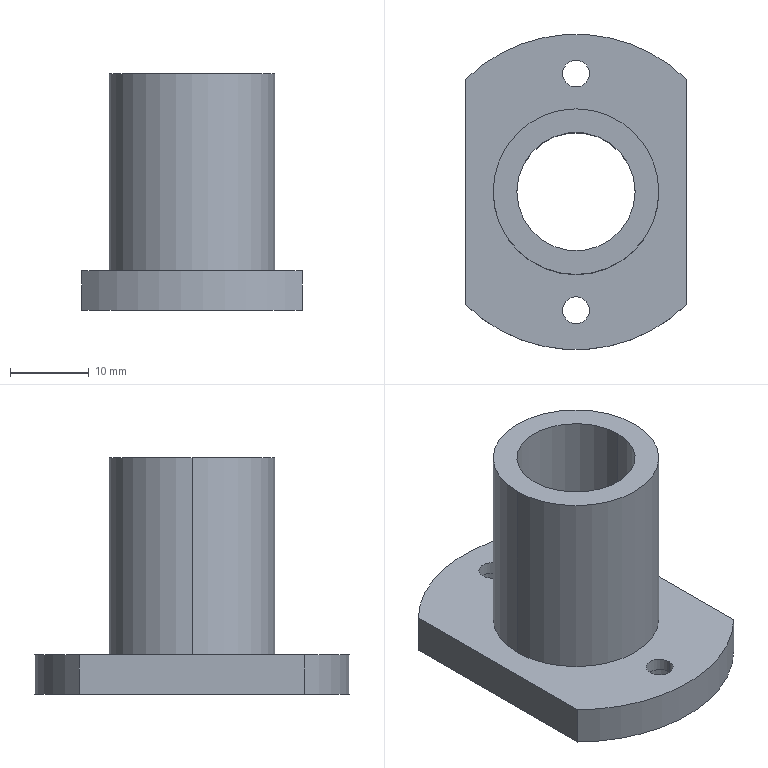Part | SolidWorks | features ICE 2, Extrusion 1, HoleWzd 1 | 1 solid | 21 faces | box 28 x 40 x 30 mm | volume 8237 mm3 | cylinder 14 | plane 7 | commonest cylinder face diameters 3.4 x4 6 x4 15 x2 21 x2 40 x2
STEP:
#1=CARTESIAN_POINT('',(3.,15.,-1.6));
#2=VERTEX_POINT('',#1);
#3=CARTESIAN_POINT('',(-3.,15.,-1.6));
#4=VERTEX_POINT('',#3);
#5=CARTESIAN_POINT('',(0.,15.,-1.6));
#6=DIRECTION('',(0.,0.,-1.));
#7=DIRECTION('',(-1.,0.,0.));
#8=AXIS2_PLACEMENT_3D('',#5,#6,#7);
#9=CIRCLE('',#8,3.);
#10=EDGE_CURVE('',#2,#4,#9,.T.);
#11=ORIENTED_EDGE('',*,*,#10,.F.);
#12=CARTESIAN_POINT('',(3.,15.,-5.));
#13=VERTEX_POINT('',#12);
#14=CARTESIAN_POINT('',(3.,15.,-5.));
#15=DIRECTION('',(0.,0.,-1.));
#16=VECTOR('',#15,1000.);
#17=LINE('',#14,#16);
#18=EDGE_CURVE('',#2,#13,#17,.T.);
#19=ORIENTED_EDGE('',*,*,#18,.T.);
#20=CARTESIAN_POINT('',(-3.,15.,-5.));
#21=VERTEX_POINT('',#20);
#22=CARTESIAN_POINT('',(0.,15.,-5.));
#23=DIRECTION('',(0.,0.,-1.));
#24=DIRECTION('',(-1.,0.,0.));
#25=AXIS2_PLACEMENT_3D('',#22,#23,#24);
#26=CIRCLE('',#25,3.);
#27=EDGE_CURVE('',#13,#21,#26,.T.);
#28=ORIENTED_EDGE('',*,*,#27,.T.);
#29=CARTESIAN_POINT('',(-3.,15.,-5.));
#30=DIRECTION('',(0.,0.,-1.));
#31=VECTOR('',#30,1000.);
#32=LINE('',#29,#31);
#33=EDGE_CURVE('',#4,#21,#32,.T.);
#34=ORIENTED_EDGE('',*,*,#33,.F.);
#35=EDGE_LOOP('',(#11,#19,#28,#34));
#36=FACE_OUTER_BOUND('',#35,.T.);
#37=CARTESIAN_POINT('',(0.,15.,-5.));
#38=DIRECTION('',(0.,0.,-1.));
#39=DIRECTION('',(-1.,0.,0.));
#40=AXIS2_PLACEMENT_3D('',#37,#38,#39);
#41=CYLINDRICAL_SURFACE('',#40,3.);
#42=ADVANCED_FACE('',(#36),#41,.F.);
#43=CARTESIAN_POINT('',(1.7,15.,0.));
#44=VERTEX_POINT('',#43);
#45=CARTESIAN_POINT('',(-1.7,15.,0.));
#46=VERTEX_POINT('',#45);
#47=CARTESIAN_POINT('',(0.,15.,0.));
#48=DIRECTION('',(0.,0.,-1.));
#49=DIRECTION('',(-1.,0.,0.));
#50=AXIS2_PLACEMENT_3D('',#47,#48,#49);
#51=CIRCLE('',#50,1.7);
#52=EDGE_CURVE('',#44,#46,#51,.T.);
#53=ORIENTED_EDGE('',*,*,#52,.F.);
#54=CARTESIAN_POINT('',(1.7,15.,-1.6));
#55=VERTEX_POINT('',#54);
#56=CARTESIAN_POINT('',(1.7,15.,-5.));
#57=DIRECTION('',(0.,0.,-1.));
#58=VECTOR('',#57,1000.);
#59=LINE('',#56,#58);
#60=EDGE_CURVE('',#44,#55,#59,.T.);
#61=ORIENTED_EDGE('',*,*,#60,.T.);
#62=CARTESIAN_POINT('',(-1.7,15.,-1.6));
#63=VERTEX_POINT('',#62);
#64=CARTESIAN_POINT('',(0.,15.,-1.6));
#65=DIRECTION('',(0.,0.,-1.));
#66=DIRECTION('',(-1.,0.,0.));
#67=AXIS2_PLACEMENT_3D('',#64,#65,#66);
#68=CIRCLE('',#67,1.7);
#69=EDGE_CURVE('',#55,#63,#68,.T.);
#70=ORIENTED_EDGE('',*,*,#69,.T.);
#71=CARTESIAN_POINT('',(-1.7,15.,-5.));
#72=DIRECTION('',(0.,0.,-1.));
#73=VECTOR('',#72,1000.);
#74=LINE('',#71,#73);
#75=EDGE_CURVE('',#46,#63,#74,.T.);
#76=ORIENTED_EDGE('',*,*,#75,.F.);
#77=EDGE_LOOP('',(#53,#61,#70,#76));
#78=FACE_OUTER_BOUND('',#77,.T.);
#79=CARTESIAN_POINT('',(0.,15.,-5.));
#80=DIRECTION('',(0.,0.,-1.));
#81=DIRECTION('',(-1.,0.,0.));
#82=AXIS2_PLACEMENT_3D('',#79,#80,#81);
#83=CYLINDRICAL_SURFACE('',#82,1.7);
#84=ADVANCED_FACE('',(#78),#83,.F.);
#85=CARTESIAN_POINT('',(3.,-15.,-1.6));
#86=VERTEX_POINT('',#85);
#87=CARTESIAN_POINT('',(-3.,-15.,-1.6));
#88=VERTEX_POINT('',#87);
#89=CARTESIAN_POINT('',(0.,-15.,-1.6));
#90=DIRECTION('',(0.,0.,-1.));
#91=DIRECTION('',(-1.,0.,0.));
#92=AXIS2_PLACEMENT_3D('',#89,#90,#91);
#93=CIRCLE('',#92,3.);
#94=EDGE_CURVE('',#86,#88,#93,.T.);
#95=ORIENTED_EDGE('',*,*,#94,.F.);
#96=CARTESIAN_POINT('',(3.,-15.,-5.));
#97=VERTEX_POINT('',#96);
#98=CARTESIAN_POINT('',(3.,-15.,-5.));
#99=DIRECTION('',(0.,0.,-1.));
#100=VECTOR('',#99,1000.);
#101=LINE('',#98,#100);
#102=EDGE_CURVE('',#86,#97,#101,.T.);
#103=ORIENTED_EDGE('',*,*,#102,.T.);
#104=CARTESIAN_POINT('',(-3.,-15.,-5.));
#105=VERTEX_POINT('',#104);
#106=CARTESIAN_POINT('',(0.,-15.,-5.));
#107=DIRECTION('',(0.,0.,-1.));
#108=DIRECTION('',(-1.,0.,0.));
#109=AXIS2_PLACEMENT_3D('',#106,#107,#108);
#110=CIRCLE('',#109,3.);
#111=EDGE_CURVE('',#97,#105,#110,.T.);
#112=ORIENTED_EDGE('',*,*,#111,.T.);
#113=CARTESIAN_POINT('',(-3.,-15.,-5.));
#114=DIRECTION('',(0.,0.,-1.));
#115=VECTOR('',#114,1000.);
#116=LINE('',#113,#115);
#117=EDGE_CURVE('',#88,#105,#116,.T.);
#118=ORIENTED_EDGE('',*,*,#117,.F.);
#119=EDGE_LOOP('',(#95,#103,#112,#118));
#120=FACE_OUTER_BOUND('',#119,.T.);
#121=CARTESIAN_POINT('',(0.,-15.,-5.));
#122=DIRECTION('',(0.,0.,-1.));
#123=DIRECTION('',(-1.,0.,0.));
#124=AXIS2_PLACEMENT_3D('',#121,#122,#123);
#125=CYLINDRICAL_SURFACE('',#124,3.);
#126=ADVANCED_FACE('',(#120),#125,.F.);
#127=CARTESIAN_POINT('',(1.7,-15.,0.));
#128=VERTEX_POINT('',#127);
#129=CARTESIAN_POINT('',(-1.7,-15.,0.));
#130=VERTEX_POINT('',#129);
#131=CARTESIAN_POINT('',(0.,-15.,0.));
#132=DIRECTION('',(0.,0.,-1.));
#133=DIRECTION('',(-1.,0.,0.));
#134=AXIS2_PLACEMENT_3D('',#131,#132,#133);
#135=CIRCLE('',#134,1.7);
#136=EDGE_CURVE('',#128,#130,#135,.T.);
#137=ORIENTED_EDGE('',*,*,#136,.F.);
#138=CARTESIAN_POINT('',(1.7,-15.,-1.6));
#139=VERTEX_POINT('',#138);
#140=CARTESIAN_POINT('',(1.7,-15.,-5.));
#141=DIRECTION('',(0.,0.,-1.));
#142=VECTOR('',#141,1000.);
#143=LINE('',#140,#142);
#144=EDGE_CURVE('',#128,#139,#143,.T.);
#145=ORIENTED_EDGE('',*,*,#144,.T.);
#146=CARTESIAN_POINT('',(-1.7,-15.,-1.6));
#147=VERTEX_POINT('',#146);
#148=CARTESIAN_POINT('',(0.,-15.,-1.6));
#149=DIRECTION('',(0.,0.,-1.));
#150=DIRECTION('',(-1.,0.,0.));
#151=AXIS2_PLACEMENT_3D('',#148,#149,#150);
#152=CIRCLE('',#151,1.7);
#153=EDGE_CURVE('',#139,#147,#152,.T.);
#154=ORIENTED_EDGE('',*,*,#153,.T.);
#155=CARTESIAN_POINT('',(-1.7,-15.,-5.));
#156=DIRECTION('',(0.,0.,-1.));
#157=VECTOR('',#156,1000.);
#158=LINE('',#155,#157);
#159=EDGE_CURVE('',#130,#147,#158,.T.);
#160=ORIENTED_EDGE('',*,*,#159,.F.);
#161=EDGE_LOOP('',(#137,#145,#154,#160));
#162=FACE_OUTER_BOUND('',#161,.T.);
#163=CARTESIAN_POINT('',(0.,-15.,-5.));
#164=DIRECTION('',(0.,0.,-1.));
#165=DIRECTION('',(-1.,0.,0.));
#166=AXIS2_PLACEMENT_3D('',#163,#164,#165);
#167=CYLINDRICAL_SURFACE('',#166,1.7);
#168=ADVANCED_FACE('',(#162),#167,.F.);
#169=CARTESIAN_POINT('',(-7.5,0.,25.));
#170=VERTEX_POINT('',#169);
#171=CARTESIAN_POINT('',(7.5,0.,25.));
#172=VERTEX_POINT('',#171);
#173=CARTESIAN_POINT('',(0.,0.,25.));
#174=DIRECTION('',(0.,0.,1.));
#175=DIRECTION('',(1.,0.,0.));
#176=AXIS2_PLACEMENT_3D('',#173,#174,#175);
#177=CIRCLE('',#176,7.5);
#178=EDGE_CURVE('',#170,#172,#177,.T.);
#179=ORIENTED_EDGE('',*,*,#178,.T.);
#180=CARTESIAN_POINT('',(7.5,0.,-5.));
#181=VERTEX_POINT('',#180);
#182=CARTESIAN_POINT('',(7.5,0.,25.));
#183=DIRECTION('',(0.,0.,-1.));
#184=VECTOR('',#183,1000.);
#185=LINE('',#182,#184);
#186=EDGE_CURVE('',#172,#181,#185,.T.);
#187=ORIENTED_EDGE('',*,*,#186,.T.);
#188=CARTESIAN_POINT('',(-7.5,0.,-5.));
#189=VERTEX_POINT('',#188);
#190=CARTESIAN_POINT('',(0.,0.,-5.));
#191=DIRECTION('',(0.,0.,-1.));
#192=DIRECTION('',(-1.,0.,0.));
#193=AXIS2_PLACEMENT_3D('',#190,#191,#192);
#194=CIRCLE('',#193,7.5);
#195=EDGE_CURVE('',#181,#189,#194,.T.);
#196=ORIENTED_EDGE('',*,*,#195,.T.);
#197=CARTESIAN_POINT('',(-7.5,0.,25.));
#198=DIRECTION('',(0.,0.,-1.));
#199=VECTOR('',#198,1000.);
#200=LINE('',#197,#199);
#201=EDGE_CURVE('',#170,#189,#200,.T.);
#202=ORIENTED_EDGE('',*,*,#201,.F.);
#203=EDGE_LOOP('',(#179,#187,#196,#202));
#204=FACE_OUTER_BOUND('',#203,.T.);
#205=CARTESIAN_POINT('',(0.,0.,25.));
#206=DIRECTION('',(0.,0.,-1.));
#207=DIRECTION('',(-1.,0.,0.));
#208=AXIS2_PLACEMENT_3D('',#205,#206,#207);
#209=CYLINDRICAL_SURFACE('',#208,7.5);
#210=ADVANCED_FACE('',(#204),#209,.F.);
#211=CARTESIAN_POINT('',(10.5,0.,25.));
#212=VERTEX_POINT('',#211);
#213=CARTESIAN_POINT('',(-10.5,0.,25.));
#214=VERTEX_POINT('',#213);
#215=CARTESIAN_POINT('',(0.,0.,25.));
#216=DIRECTION('',(0.,0.,1.));
#217=DIRECTION('',(1.,0.,0.));
#218=AXIS2_PLACEMENT_3D('',#215,#216,#217);
#219=CIRCLE('',#218,10.5);
#220=EDGE_CURVE('',#212,#214,#219,.T.);
#221=ORIENTED_EDGE('',*,*,#220,.F.);
#222=CARTESIAN_POINT('',(10.5,0.,0.));
#223=VERTEX_POINT('',#222);
#224=CARTESIAN_POINT('',(10.5,0.,25.));
#225=DIRECTION('',(0.,0.,-1.));
#226=VECTOR('',#225,1000.);
#227=LINE('',#224,#226);
#228=EDGE_CURVE('',#212,#223,#227,.T.);
#229=ORIENTED_EDGE('',*,*,#228,.T.);
#230=CARTESIAN_POINT('',(-10.5,0.,0.));
#231=VERTEX_POINT('',#230);
#232=CARTESIAN_POINT('',(0.,0.,0.));
#233=DIRECTION('',(0.,0.,-1.));
#234=DIRECTION('',(-1.,0.,0.));
#235=AXIS2_PLACEMENT_3D('',#232,#233,#234);
#236=CIRCLE('',#235,10.5);
#237=EDGE_CURVE('',#231,#223,#236,.T.);
#238=ORIENTED_EDGE('',*,*,#237,.F.);
#239=CARTESIAN_POINT('',(-10.5,0.,25.));
#240=DIRECTION('',(0.,0.,-1.));
#241=VECTOR('',#240,1000.);
#242=LINE('',#239,#241);
#243=EDGE_CURVE('',#214,#231,#242,.T.);
#244=ORIENTED_EDGE('',*,*,#243,.F.);
#245=EDGE_LOOP('',(#221,#229,#238,#244));
#246=FACE_OUTER_BOUND('',#245,.T.);
#247=CARTESIAN_POINT('',(0.,0.,25.));
#248=DIRECTION('',(0.,0.,-1.));
#249=DIRECTION('',(-1.,0.,0.));
#250=AXIS2_PLACEMENT_3D('',#247,#248,#249);
#251=CYLINDRICAL_SURFACE('',#250,10.5);
#252=ADVANCED_FACE('',(#246),#251,.T.);
#253=CARTESIAN_POINT('',(-14.,14.283,-5.));
#254=VERTEX_POINT('',#253);
#255=CARTESIAN_POINT('',(14.,14.283,-5.));
#256=VERTEX_POINT('',#255);
#257=CARTESIAN_POINT('',(0.,0.,-5.));
#258=DIRECTION('',(0.,0.,-1.));
#259=DIRECTION('',(-1.,0.,0.));
#260=AXIS2_PLACEMENT_3D('',#257,#258,#259);
#261=CIRCLE('',#260,20.);
#262=EDGE_CURVE('',#254,#256,#261,.T.);
#263=ORIENTED_EDGE('',*,*,#262,.F.);
#264=CARTESIAN_POINT('',(-14.,14.283,0.));
#265=VERTEX_POINT('',#264);
#266=CARTESIAN_POINT('',(-14.,14.283,-5.));
#267=DIRECTION('',(0.,0.,1.));
#268=VECTOR('',#267,1000.);
#269=LINE('',#266,#268);
#270=EDGE_CURVE('',#254,#265,#269,.T.);
#271=ORIENTED_EDGE('',*,*,#270,.T.);
#272=CARTESIAN_POINT('',(14.,14.283,0.));
#273=VERTEX_POINT('',#272);
#274=CARTESIAN_POINT('',(0.,0.,0.));
#275=DIRECTION('',(0.,0.,-1.));
#276=DIRECTION('',(-1.,0.,0.));
#277=AXIS2_PLACEMENT_3D('',#274,#275,#276);
#278=CIRCLE('',#277,20.);
#279=EDGE_CURVE('',#265,#273,#278,.T.);
#280=ORIENTED_EDGE('',*,*,#279,.T.);
#281=CARTESIAN_POINT('',(14.,14.283,-5.));
#282=DIRECTION('',(0.,0.,-1.));
#283=VECTOR('',#282,1000.);
#284=LINE('',#281,#283);
#285=EDGE_CURVE('',#273,#256,#284,.T.);
#286=ORIENTED_EDGE('',*,*,#285,.T.);
#287=EDGE_LOOP('',(#263,#271,#280,#286));
#288=FACE_OUTER_BOUND('',#287,.T.);
#289=CARTESIAN_POINT('',(0.,0.,-5.));
#290=DIRECTION('',(0.,0.,1.));
#291=DIRECTION('',(1.,0.,0.));
#292=AXIS2_PLACEMENT_3D('',#289,#290,#291);
#293=CYLINDRICAL_SURFACE('',#292,20.);
#294=ADVANCED_FACE('',(#288),#293,.T.);
#295=CARTESIAN_POINT('',(0.,0.,25.));
#296=DIRECTION('',(0.,0.,1.));
#297=DIRECTION('',(1.,0.,0.));
#298=AXIS2_PLACEMENT_3D('',#295,#296,#297);
#299=CIRCLE('',#298,10.5);
#300=EDGE_CURVE('',#214,#212,#299,.T.);
#301=ORIENTED_EDGE('',*,*,#300,.T.);
#302=ORIENTED_EDGE('',*,*,#220,.T.);
#303=EDGE_LOOP('',(#301,#302));
#304=FACE_OUTER_BOUND('',#303,.T.);
#305=ORIENTED_EDGE('',*,*,#178,.F.);
#306=CARTESIAN_POINT('',(0.,0.,25.));
#307=DIRECTION('',(0.,0.,1.));
#308=DIRECTION('',(1.,0.,0.));
#309=AXIS2_PLACEMENT_3D('',#306,#307,#308);
#310=CIRCLE('',#309,7.5);
#311=EDGE_CURVE('',#172,#170,#310,.T.);
#312=ORIENTED_EDGE('',*,*,#311,.F.);
#313=EDGE_LOOP('',(#305,#312));
#314=FACE_BOUND('',#313,.T.);
#315=CARTESIAN_POINT('',(0.,0.,25.));
#316=DIRECTION('',(0.,0.,1.));
#317=DIRECTION('',(1.,0.,0.));
#318=AXIS2_PLACEMENT_3D('',#315,#316,#317);
#319=PLANE('',#318);
#320=ADVANCED_FACE('',(#304,#314),#319,.T.);
#321=ORIENTED_EDGE('',*,*,#228,.F.);
#322=ORIENTED_EDGE('',*,*,#300,.F.);
#323=ORIENTED_EDGE('',*,*,#243,.T.);
#324=CARTESIAN_POINT('',(0.,0.,0.));
#325=DIRECTION('',(0.,0.,-1.));
#326=DIRECTION('',(-1.,0.,0.));
#327=AXIS2_PLACEMENT_3D('',#324,#325,#326);
#328=CIRCLE('',#327,10.5);
#329=EDGE_CURVE('',#223,#231,#328,.T.);
#330=ORIENTED_EDGE('',*,*,#329,.F.);
#331=EDGE_LOOP('',(#321,#322,#323,#330));
#332=FACE_OUTER_BOUND('',#331,.T.);
#333=CARTESIAN_POINT('',(0.,0.,25.));
#334=DIRECTION('',(0.,0.,-1.));
#335=DIRECTION('',(-1.,0.,0.));
#336=AXIS2_PLACEMENT_3D('',#333,#334,#335);
#337=CYLINDRICAL_SURFACE('',#336,10.5);
#338=ADVANCED_FACE('',(#332),#337,.T.);
#339=ORIENTED_EDGE('',*,*,#186,.F.);
#340=ORIENTED_EDGE('',*,*,#311,.T.);
#341=ORIENTED_EDGE('',*,*,#201,.T.);
#342=CARTESIAN_POINT('',(0.,0.,-5.));
#343=DIRECTION('',(0.,0.,-1.));
#344=DIRECTION('',(-1.,0.,0.));
#345=AXIS2_PLACEMENT_3D('',#342,#343,#344);
#346=CIRCLE('',#345,7.5);
#347=EDGE_CURVE('',#189,#181,#346,.T.);
#348=ORIENTED_EDGE('',*,*,#347,.T.);
#349=EDGE_LOOP('',(#339,#340,#341,#348));
#350=FACE_OUTER_BOUND('',#349,.T.);
#351=CARTESIAN_POINT('',(0.,0.,25.));
#352=DIRECTION('',(0.,0.,-1.));
#353=DIRECTION('',(-1.,0.,0.));
#354=AXIS2_PLACEMENT_3D('',#351,#352,#353);
#355=CYLINDRICAL_SURFACE('',#354,7.5);
#356=ADVANCED_FACE('',(#350),#355,.F.);
#357=CARTESIAN_POINT('',(0.,15.,0.));
#358=DIRECTION('',(0.,0.,-1.));
#359=DIRECTION('',(-1.,0.,0.));
#360=AXIS2_PLACEMENT_3D('',#357,#358,#359);
#361=CIRCLE('',#360,1.7);
#362=EDGE_CURVE('',#46,#44,#361,.T.);
#363=ORIENTED_EDGE('',*,*,#362,.T.);
#364=ORIENTED_EDGE('',*,*,#52,.T.);
#365=EDGE_LOOP('',(#363,#364));
#366=FACE_BOUND('',#365,.T.);
#367=CARTESIAN_POINT('',(0.,-15.,0.));
#368=DIRECTION('',(0.,0.,-1.));
#369=DIRECTION('',(-1.,0.,0.));
#370=AXIS2_PLACEMENT_3D('',#367,#368,#369);
#371=CIRCLE('',#370,1.7);
#372=EDGE_CURVE('',#130,#128,#371,.T.);
#373=ORIENTED_EDGE('',*,*,#372,.T.);
#374=ORIENTED_EDGE('',*,*,#136,.T.);
#375=EDGE_LOOP('',(#373,#374));
#376=FACE_BOUND('',#375,.T.);
#377=ORIENTED_EDGE('',*,*,#279,.F.);
#378=CARTESIAN_POINT('',(-14.,-14.283,0.));
#379=VERTEX_POINT('',#378);
#380=CARTESIAN_POINT('',(-14.,0.,0.));
#381=DIRECTION('',(0.,-1.,0.));
#382=VECTOR('',#381,1000.);
#383=LINE('',#380,#382);
#384=EDGE_CURVE('',#265,#379,#383,.T.);
#385=ORIENTED_EDGE('',*,*,#384,.T.);
#386=CARTESIAN_POINT('',(14.,-14.283,0.));
#387=VERTEX_POINT('',#386);
#388=CARTESIAN_POINT('',(0.,0.,0.));
#389=DIRECTION('',(0.,0.,-1.));
#390=DIRECTION('',(-1.,0.,0.));
#391=AXIS2_PLACEMENT_3D('',#388,#389,#390);
#392=CIRCLE('',#391,20.);
#393=EDGE_CURVE('',#387,#379,#392,.T.);
#394=ORIENTED_EDGE('',*,*,#393,.F.);
#395=CARTESIAN_POINT('',(14.,0.,0.));
#396=DIRECTION('',(0.,1.,0.));
#397=VECTOR('',#396,1000.);
#398=LINE('',#395,#397);
#399=EDGE_CURVE('',#387,#273,#398,.T.);
#400=ORIENTED_EDGE('',*,*,#399,.T.);
#401=EDGE_LOOP('',(#377,#385,#394,#400));
#402=FACE_OUTER_BOUND('',#401,.T.);
#403=ORIENTED_EDGE('',*,*,#237,.T.);
#404=ORIENTED_EDGE('',*,*,#329,.T.);
#405=EDGE_LOOP('',(#403,#404));
#406=FACE_BOUND('',#405,.T.);
#407=CARTESIAN_POINT('',(0.,0.,0.));
#408=DIRECTION('',(0.,0.,-1.));
#409=DIRECTION('',(-1.,0.,0.));
#410=AXIS2_PLACEMENT_3D('',#407,#408,#409);
#411=PLANE('',#410);
#412=ADVANCED_FACE('',(#366,#376,#402,#406),#411,.F.);
#413=CARTESIAN_POINT('',(-14.,-14.283,-5.));
#414=VERTEX_POINT('',#413);
#415=CARTESIAN_POINT('',(-14.,20.486,-5.));
#416=DIRECTION('',(0.,-1.,0.));
#417=VECTOR('',#416,1000.);
#418=LINE('',#415,#417);
#419=EDGE_CURVE('',#254,#414,#418,.T.);
#420=ORIENTED_EDGE('',*,*,#419,.F.);
#421=ORIENTED_EDGE('',*,*,#262,.T.);
#422=CARTESIAN_POINT('',(14.,-14.283,-5.));
#423=VERTEX_POINT('',#422);
#424=CARTESIAN_POINT('',(14.,22.593,-5.));
#425=DIRECTION('',(0.,1.,0.));
#426=VECTOR('',#425,1000.);
#427=LINE('',#424,#426);
#428=EDGE_CURVE('',#423,#256,#427,.T.);
#429=ORIENTED_EDGE('',*,*,#428,.F.);
#430=CARTESIAN_POINT('',(0.,0.,-5.));
#431=DIRECTION('',(0.,0.,-1.));
#432=DIRECTION('',(-1.,0.,0.));
#433=AXIS2_PLACEMENT_3D('',#430,#431,#432);
#434=CIRCLE('',#433,20.);
#435=EDGE_CURVE('',#423,#414,#434,.T.);
#436=ORIENTED_EDGE('',*,*,#435,.T.);
#437=EDGE_LOOP('',(#420,#421,#429,#436));
#438=FACE_OUTER_BOUND('',#437,.T.);
#439=CARTESIAN_POINT('',(0.,15.,-5.));
#440=DIRECTION('',(0.,0.,-1.));
#441=DIRECTION('',(-1.,0.,0.));
#442=AXIS2_PLACEMENT_3D('',#439,#440,#441);
#443=CIRCLE('',#442,3.);
#444=EDGE_CURVE('',#21,#13,#443,.T.);
#445=ORIENTED_EDGE('',*,*,#444,.F.);
#446=ORIENTED_EDGE('',*,*,#27,.F.);
#447=EDGE_LOOP('',(#445,#446));
#448=FACE_BOUND('',#447,.T.);
#449=CARTESIAN_POINT('',(0.,-15.,-5.));
#450=DIRECTION('',(0.,0.,-1.));
#451=DIRECTION('',(-1.,0.,0.));
#452=AXIS2_PLACEMENT_3D('',#449,#450,#451);
#453=CIRCLE('',#452,3.);
#454=EDGE_CURVE('',#105,#97,#453,.T.);
#455=ORIENTED_EDGE('',*,*,#454,.F.);
#456=ORIENTED_EDGE('',*,*,#111,.F.);
#457=EDGE_LOOP('',(#455,#456));
#458=FACE_BOUND('',#457,.T.);
#459=ORIENTED_EDGE('',*,*,#347,.F.);
#460=ORIENTED_EDGE('',*,*,#195,.F.);
#461=EDGE_LOOP('',(#459,#460));
#462=FACE_BOUND('',#461,.T.);
#463=CARTESIAN_POINT('',(0.,0.,-5.));
#464=DIRECTION('',(0.,0.,-1.));
#465=DIRECTION('',(-1.,0.,0.));
#466=AXIS2_PLACEMENT_3D('',#463,#464,#465);
#467=PLANE('',#466);
#468=ADVANCED_FACE('',(#438,#448,#458,#462),#467,.T.);
#469=ORIENTED_EDGE('',*,*,#393,.T.);
#470=CARTESIAN_POINT('',(-14.,-14.283,-5.));
#471=DIRECTION('',(0.,0.,-1.));
#472=VECTOR('',#471,1000.);
#473=LINE('',#470,#472);
#474=EDGE_CURVE('',#379,#414,#473,.T.);
#475=ORIENTED_EDGE('',*,*,#474,.T.);
#476=ORIENTED_EDGE('',*,*,#435,.F.);
#477=CARTESIAN_POINT('',(14.,-14.283,-5.));
#478=DIRECTION('',(0.,0.,1.));
#479=VECTOR('',#478,1000.);
#480=LINE('',#477,#479);
#481=EDGE_CURVE('',#423,#387,#480,.T.);
#482=ORIENTED_EDGE('',*,*,#481,.T.);
#483=EDGE_LOOP('',(#469,#475,#476,#482));
#484=FACE_OUTER_BOUND('',#483,.T.);
#485=CARTESIAN_POINT('',(0.,0.,-5.));
#486=DIRECTION('',(0.,0.,1.));
#487=DIRECTION('',(1.,0.,0.));
#488=AXIS2_PLACEMENT_3D('',#485,#486,#487);
#489=CYLINDRICAL_SURFACE('',#488,20.);
#490=ADVANCED_FACE('',(#484),#489,.T.);
#491=ORIENTED_EDGE('',*,*,#144,.F.);
#492=ORIENTED_EDGE('',*,*,#372,.F.);
#493=ORIENTED_EDGE('',*,*,#159,.T.);
#494=CARTESIAN_POINT('',(0.,-15.,-1.6));
#495=DIRECTION('',(0.,0.,-1.));
#496=DIRECTION('',(-1.,0.,0.));
#497=AXIS2_PLACEMENT_3D('',#494,#495,#496);
#498=CIRCLE('',#497,1.7);
#499=EDGE_CURVE('',#147,#139,#498,.T.);
#500=ORIENTED_EDGE('',*,*,#499,.T.);
#501=EDGE_LOOP('',(#491,#492,#493,#500));
#502=FACE_OUTER_BOUND('',#501,.T.);
#503=CARTESIAN_POINT('',(0.,-15.,-5.));
#504=DIRECTION('',(0.,0.,-1.));
#505=DIRECTION('',(-1.,0.,0.));
#506=AXIS2_PLACEMENT_3D('',#503,#504,#505);
#507=CYLINDRICAL_SURFACE('',#506,1.7);
#508=ADVANCED_FACE('',(#502),#507,.F.);
#509=ORIENTED_EDGE('',*,*,#499,.F.);
#510=ORIENTED_EDGE('',*,*,#153,.F.);
#511=EDGE_LOOP('',(#509,#510));
#512=FACE_BOUND('',#511,.T.);
#513=CARTESIAN_POINT('',(0.,-15.,-1.6));
#514=DIRECTION('',(0.,0.,-1.));
#515=DIRECTION('',(-1.,0.,0.));
#516=AXIS2_PLACEMENT_3D('',#513,#514,#515);
#517=CIRCLE('',#516,3.);
#518=EDGE_CURVE('',#88,#86,#517,.T.);
#519=ORIENTED_EDGE('',*,*,#518,.T.);
#520=ORIENTED_EDGE('',*,*,#94,.T.);
#521=EDGE_LOOP('',(#519,#520));
#522=FACE_OUTER_BOUND('',#521,.T.);
#523=CARTESIAN_POINT('',(1.7,-15.,-1.6));
#524=DIRECTION('',(0.,0.,1.));
#525=DIRECTION('',(1.,0.,0.));
#526=AXIS2_PLACEMENT_3D('',#523,#524,#525);
#527=PLANE('',#526);
#528=ADVANCED_FACE('',(#512,#522),#527,.F.);
#529=ORIENTED_EDGE('',*,*,#102,.F.);
#530=ORIENTED_EDGE('',*,*,#518,.F.);
#531=ORIENTED_EDGE('',*,*,#117,.T.);
#532=ORIENTED_EDGE('',*,*,#454,.T.);
#533=EDGE_LOOP('',(#529,#530,#531,#532));
#534=FACE_OUTER_BOUND('',#533,.T.);
#535=CARTESIAN_POINT('',(0.,-15.,-5.));
#536=DIRECTION('',(0.,0.,-1.));
#537=DIRECTION('',(-1.,0.,0.));
#538=AXIS2_PLACEMENT_3D('',#535,#536,#537);
#539=CYLINDRICAL_SURFACE('',#538,3.);
#540=ADVANCED_FACE('',(#534),#539,.F.);
#541=ORIENTED_EDGE('',*,*,#60,.F.);
#542=ORIENTED_EDGE('',*,*,#362,.F.);
#543=ORIENTED_EDGE('',*,*,#75,.T.);
#544=CARTESIAN_POINT('',(0.,15.,-1.6));
#545=DIRECTION('',(0.,0.,-1.));
#546=DIRECTION('',(-1.,0.,0.));
#547=AXIS2_PLACEMENT_3D('',#544,#545,#546);
#548=CIRCLE('',#547,1.7);
#549=EDGE_CURVE('',#63,#55,#548,.T.);
#550=ORIENTED_EDGE('',*,*,#549,.T.);
#551=EDGE_LOOP('',(#541,#542,#543,#550));
#552=FACE_OUTER_BOUND('',#551,.T.);
#553=CARTESIAN_POINT('',(0.,15.,-5.));
#554=DIRECTION('',(0.,0.,-1.));
#555=DIRECTION('',(-1.,0.,0.));
#556=AXIS2_PLACEMENT_3D('',#553,#554,#555);
#557=CYLINDRICAL_SURFACE('',#556,1.7);
#558=ADVANCED_FACE('',(#552),#557,.F.);
#559=ORIENTED_EDGE('',*,*,#549,.F.);
#560=ORIENTED_EDGE('',*,*,#69,.F.);
#561=EDGE_LOOP('',(#559,#560));
#562=FACE_BOUND('',#561,.T.);
#563=CARTESIAN_POINT('',(0.,15.,-1.6));
#564=DIRECTION('',(0.,0.,-1.));
#565=DIRECTION('',(-1.,0.,0.));
#566=AXIS2_PLACEMENT_3D('',#563,#564,#565);
#567=CIRCLE('',#566,3.);
#568=EDGE_CURVE('',#4,#2,#567,.T.);
#569=ORIENTED_EDGE('',*,*,#568,.T.);
#570=ORIENTED_EDGE('',*,*,#10,.T.);
#571=EDGE_LOOP('',(#569,#570));
#572=FACE_OUTER_BOUND('',#571,.T.);
#573=CARTESIAN_POINT('',(1.7,15.,-1.6));
#574=DIRECTION('',(0.,0.,1.));
#575=DIRECTION('',(1.,0.,0.));
#576=AXIS2_PLACEMENT_3D('',#573,#574,#575);
#577=PLANE('',#576);
#578=ADVANCED_FACE('',(#562,#572),#577,.F.);
#579=ORIENTED_EDGE('',*,*,#18,.F.);
#580=ORIENTED_EDGE('',*,*,#568,.F.);
#581=ORIENTED_EDGE('',*,*,#33,.T.);
#582=ORIENTED_EDGE('',*,*,#444,.T.);
#583=EDGE_LOOP('',(#579,#580,#581,#582));
#584=FACE_OUTER_BOUND('',#583,.T.);
#585=CARTESIAN_POINT('',(0.,15.,-5.));
#586=DIRECTION('',(0.,0.,-1.));
#587=DIRECTION('',(-1.,0.,0.));
#588=AXIS2_PLACEMENT_3D('',#585,#586,#587);
#589=CYLINDRICAL_SURFACE('',#588,3.);
#590=ADVANCED_FACE('',(#584),#589,.F.);
#591=ORIENTED_EDGE('',*,*,#428,.T.);
#592=ORIENTED_EDGE('',*,*,#285,.F.);
#593=ORIENTED_EDGE('',*,*,#399,.F.);
#594=ORIENTED_EDGE('',*,*,#481,.F.);
#595=EDGE_LOOP('',(#591,#592,#593,#594));
#596=FACE_OUTER_BOUND('',#595,.T.);
#597=CARTESIAN_POINT('',(14.,22.593,5.));
#598=DIRECTION('',(-1.,0.,0.));
#599=DIRECTION('',(0.,-1.,0.));
#600=AXIS2_PLACEMENT_3D('',#597,#598,#599);
#601=PLANE('',#600);
#602=ADVANCED_FACE('',(#596),#601,.F.);
#603=ORIENTED_EDGE('',*,*,#419,.T.);
#604=ORIENTED_EDGE('',*,*,#474,.F.);
#605=ORIENTED_EDGE('',*,*,#384,.F.);
#606=ORIENTED_EDGE('',*,*,#270,.F.);
#607=EDGE_LOOP('',(#603,#604,#605,#606));
#608=FACE_OUTER_BOUND('',#607,.T.);
#609=CARTESIAN_POINT('',(-14.,20.486,5.));
#610=DIRECTION('',(1.,0.,0.));
#611=DIRECTION('',(0.,1.,0.));
#612=AXIS2_PLACEMENT_3D('',#609,#610,#611);
#613=PLANE('',#612);
#614=ADVANCED_FACE('',(#608),#613,.F.);
#615=CLOSED_SHELL('',(#42,#84,#126,#168,#210,#252,#294,#320,#338,#356,#412,#468,#490,#508,#528,#540,#558,#578,#590,#602,#614));
#616=MANIFOLD_SOLID_BREP('',#615);
#617=CARTESIAN_POINT('',(0.,0.,0.));
#618=DIRECTION('',(0.,0.,1.));
#619=DIRECTION('',(1.,0.,0.));
#620=AXIS2_PLACEMENT_3D('',#617,#618,#619);
#621=(LENGTH_UNIT()NAMED_UNIT(*)SI_UNIT(.MILLI.,.METRE.));
#622=UNCERTAINTY_MEASURE_WITH_UNIT(LENGTH_MEASURE(0.00001),#621,'','');
#623=(NAMED_UNIT(*)PLANE_ANGLE_UNIT()SI_UNIT($,.RADIAN.));
#624=(NAMED_UNIT(*)SI_UNIT($,.STERADIAN.)SOLID_ANGLE_UNIT());
#625=(GEOMETRIC_REPRESENTATION_CONTEXT(3)GLOBAL_UNCERTAINTY_ASSIGNED_CONTEXT((#622))GLOBAL_UNIT_ASSIGNED_CONTEXT((#621,#623,#624))REPRESENTATION_CONTEXT('',''));
#626=ADVANCED_BREP_SHAPE_REPRESENTATION('',(#616,#620),#625);